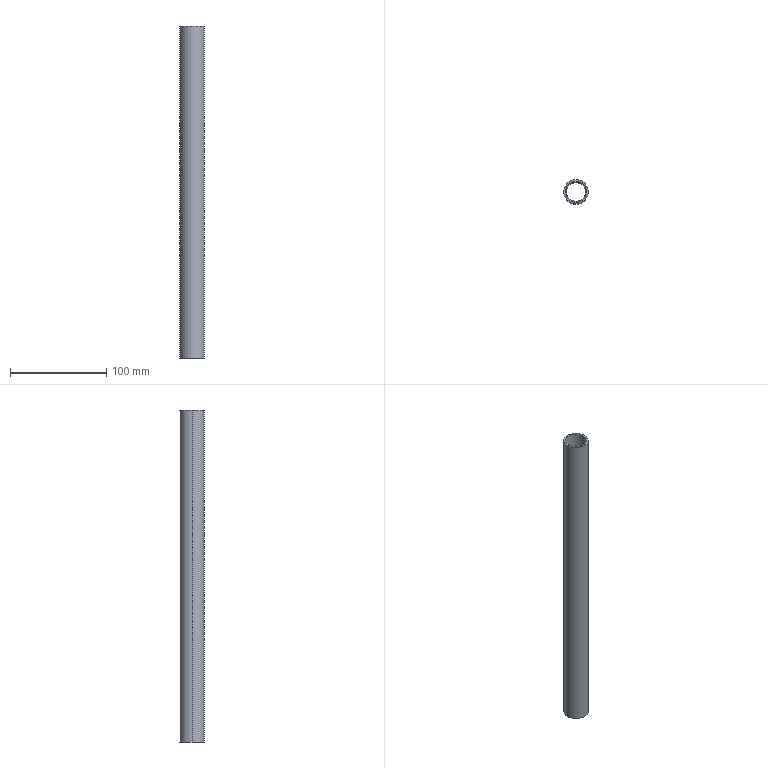Part | STEP file | 31E-01006QY25 | 1 solid | 12 faces | box 25.4 x 25.4 x 345 mm | volume 60669 mm3 | cylinder 8 | plane 4 | commonest cylinder face diameters 22.2 x4 19.8 x2 25.4 x2
STEP:
#1=CARTESIAN_POINT('',(12.7,0.,0.));
#2=VERTEX_POINT('',#1);
#3=CARTESIAN_POINT('',(12.7,0.,345.));
#4=VERTEX_POINT('',#3);
#5=CARTESIAN_POINT('',(12.7,0.,172.5));
#6=DIRECTION('',(0.,0.,1.));
#7=VECTOR('',#6,1.);
#8=LINE('',#5,#7);
#9=EDGE_CURVE('',#2,#4,#8,.T.);
#10=ORIENTED_EDGE('',*,*,#9,.F.);
#11=CARTESIAN_POINT('',(-12.7,0.,0.));
#12=VERTEX_POINT('',#11);
#13=CARTESIAN_POINT('',(0.,0.,0.));
#14=DIRECTION('',(0.,0.,1.));
#15=AXIS2_PLACEMENT_3D('',#13,#14,$);
#16=CIRCLE('',#15,12.7);
#17=EDGE_CURVE('',#2,#12,#16,.T.);
#18=ORIENTED_EDGE('',*,*,#17,.T.);
#19=CARTESIAN_POINT('',(-12.7,0.,345.));
#20=VERTEX_POINT('',#19);
#21=CARTESIAN_POINT('',(-12.7,0.,172.5));
#22=DIRECTION('',(0.,0.,1.));
#23=VECTOR('',#22,1.);
#24=LINE('',#21,#23);
#25=EDGE_CURVE('',#12,#20,#24,.T.);
#26=ORIENTED_EDGE('',*,*,#25,.T.);
#27=CARTESIAN_POINT('',(0.,0.,345.));
#28=DIRECTION('',(0.,0.,1.));
#29=AXIS2_PLACEMENT_3D('',#27,#28,$);
#30=CIRCLE('',#29,12.7);
#31=EDGE_CURVE('',#4,#20,#30,.T.);
#32=ORIENTED_EDGE('',*,*,#31,.F.);
#33=EDGE_LOOP('',(#10,#18,#26,#32));
#34=FACE_OUTER_BOUND('',#33,.T.);
#35=CARTESIAN_POINT('',(0.,0.,172.5));
#36=DIRECTION('',(0.,0.,1.));
#37=DIRECTION('',(1.,0.,0.));
#38=AXIS2_PLACEMENT_3D('',#35,#36,#37);
#39=CYLINDRICAL_SURFACE('',#38,12.7);
#40=ADVANCED_FACE('',(#34),#39,.T.);
#41=ORIENTED_EDGE('',*,*,#25,.F.);
#42=CARTESIAN_POINT('',(0.,0.,0.));
#43=DIRECTION('',(0.,0.,1.));
#44=AXIS2_PLACEMENT_3D('',#42,#43,$);
#45=CIRCLE('',#44,12.7);
#46=EDGE_CURVE('',#12,#2,#45,.T.);
#47=ORIENTED_EDGE('',*,*,#46,.T.);
#48=ORIENTED_EDGE('',*,*,#9,.T.);
#49=CARTESIAN_POINT('',(0.,0.,345.));
#50=DIRECTION('',(0.,0.,1.));
#51=AXIS2_PLACEMENT_3D('',#49,#50,$);
#52=CIRCLE('',#51,12.7);
#53=EDGE_CURVE('',#20,#4,#52,.T.);
#54=ORIENTED_EDGE('',*,*,#53,.F.);
#55=EDGE_LOOP('',(#41,#47,#48,#54));
#56=FACE_OUTER_BOUND('',#55,.T.);
#57=ADVANCED_FACE('',(#56),#39,.T.);
#58=ORIENTED_EDGE('',*,*,#31,.T.);
#59=ORIENTED_EDGE('',*,*,#53,.T.);
#60=EDGE_LOOP('',(#58,#59));
#61=FACE_OUTER_BOUND('',#60,.T.);
#62=CARTESIAN_POINT('',(11.1,0.,345.));
#63=VERTEX_POINT('',#62);
#64=CARTESIAN_POINT('',(-11.1,0.,345.));
#65=VERTEX_POINT('',#64);
#66=CARTESIAN_POINT('',(0.,0.,345.));
#67=DIRECTION('',(0.,0.,1.));
#68=AXIS2_PLACEMENT_3D('',#66,#67,$);
#69=CIRCLE('',#68,11.1);
#70=EDGE_CURVE('',#63,#65,#69,.T.);
#71=ORIENTED_EDGE('',*,*,#70,.F.);
#72=CARTESIAN_POINT('',(0.,0.,345.));
#73=DIRECTION('',(0.,0.,1.));
#74=AXIS2_PLACEMENT_3D('',#72,#73,$);
#75=CIRCLE('',#74,11.1);
#76=EDGE_CURVE('',#65,#63,#75,.T.);
#77=ORIENTED_EDGE('',*,*,#76,.F.);
#78=EDGE_LOOP('',(#71,#77));
#79=FACE_BOUND('',#78,.T.);
#80=CARTESIAN_POINT('',(0.,0.,345.));
#81=DIRECTION('',(0.,0.,1.));
#82=DIRECTION('',(1.,0.,0.));
#83=AXIS2_PLACEMENT_3D('',#80,#81,#82);
#84=PLANE('',#83);
#85=ADVANCED_FACE('',(#61,#79),#84,.T.);
#86=CARTESIAN_POINT('',(11.1,0.,295.));
#87=VERTEX_POINT('',#86);
#88=CARTESIAN_POINT('',(11.1,0.,172.5));
#89=DIRECTION('',(0.,0.,1.));
#90=VECTOR('',#89,1.);
#91=LINE('',#88,#90);
#92=EDGE_CURVE('',#63,#87,#91,.F.);
#93=ORIENTED_EDGE('',*,*,#92,.F.);
#94=ORIENTED_EDGE('',*,*,#70,.T.);
#95=CARTESIAN_POINT('',(-11.1,0.,295.));
#96=VERTEX_POINT('',#95);
#97=CARTESIAN_POINT('',(-11.1,0.,172.5));
#98=DIRECTION('',(0.,0.,1.));
#99=VECTOR('',#98,1.);
#100=LINE('',#97,#99);
#101=EDGE_CURVE('',#65,#96,#100,.F.);
#102=ORIENTED_EDGE('',*,*,#101,.T.);
#103=CARTESIAN_POINT('',(0.,0.,295.));
#104=DIRECTION('',(0.,0.,1.));
#105=AXIS2_PLACEMENT_3D('',#103,#104,$);
#106=CIRCLE('',#105,11.1);
#107=EDGE_CURVE('',#87,#96,#106,.T.);
#108=ORIENTED_EDGE('',*,*,#107,.F.);
#109=EDGE_LOOP('',(#93,#94,#102,#108));
#110=FACE_OUTER_BOUND('',#109,.T.);
#111=CARTESIAN_POINT('',(0.,0.,320.));
#112=DIRECTION('',(0.,0.,1.));
#113=DIRECTION('',(1.,0.,0.));
#114=AXIS2_PLACEMENT_3D('',#111,#112,#113);
#115=CYLINDRICAL_SURFACE('',#114,11.1);
#116=ADVANCED_FACE('',(#110),#115,.F.);
#117=ORIENTED_EDGE('',*,*,#101,.F.);
#118=ORIENTED_EDGE('',*,*,#76,.T.);
#119=ORIENTED_EDGE('',*,*,#92,.T.);
#120=CARTESIAN_POINT('',(0.,0.,295.));
#121=DIRECTION('',(0.,0.,1.));
#122=AXIS2_PLACEMENT_3D('',#120,#121,$);
#123=CIRCLE('',#122,11.1);
#124=EDGE_CURVE('',#96,#87,#123,.T.);
#125=ORIENTED_EDGE('',*,*,#124,.F.);
#126=EDGE_LOOP('',(#117,#118,#119,#125));
#127=FACE_OUTER_BOUND('',#126,.T.);
#128=ADVANCED_FACE('',(#127),#115,.F.);
#129=ORIENTED_EDGE('',*,*,#107,.T.);
#130=ORIENTED_EDGE('',*,*,#124,.T.);
#131=EDGE_LOOP('',(#129,#130));
#132=FACE_OUTER_BOUND('',#131,.T.);
#133=CARTESIAN_POINT('',(-9.9,0.,295.));
#134=VERTEX_POINT('',#133);
#135=CARTESIAN_POINT('',(9.9,0.,295.));
#136=VERTEX_POINT('',#135);
#137=CARTESIAN_POINT('',(0.,0.,295.));
#138=DIRECTION('',(0.,0.,1.));
#139=AXIS2_PLACEMENT_3D('',#137,#138,$);
#140=CIRCLE('',#139,9.9);
#141=EDGE_CURVE('',#134,#136,#140,.T.);
#142=ORIENTED_EDGE('',*,*,#141,.F.);
#143=CARTESIAN_POINT('',(0.,0.,295.));
#144=DIRECTION('',(0.,0.,1.));
#145=AXIS2_PLACEMENT_3D('',#143,#144,$);
#146=CIRCLE('',#145,9.9);
#147=EDGE_CURVE('',#136,#134,#146,.T.);
#148=ORIENTED_EDGE('',*,*,#147,.F.);
#149=EDGE_LOOP('',(#142,#148));
#150=FACE_BOUND('',#149,.T.);
#151=CARTESIAN_POINT('',(0.,0.,295.));
#152=DIRECTION('',(0.,0.,1.));
#153=DIRECTION('',(1.,0.,0.));
#154=AXIS2_PLACEMENT_3D('',#151,#152,#153);
#155=PLANE('',#154);
#156=ADVANCED_FACE('',(#132,#150),#155,.T.);
#157=CARTESIAN_POINT('',(-9.9,0.,50.));
#158=VERTEX_POINT('',#157);
#159=CARTESIAN_POINT('',(9.9,0.,50.));
#160=VERTEX_POINT('',#159);
#161=CARTESIAN_POINT('',(0.,0.,50.));
#162=DIRECTION('',(0.,0.,1.));
#163=AXIS2_PLACEMENT_3D('',#161,#162,$);
#164=CIRCLE('',#163,9.9);
#165=EDGE_CURVE('',#158,#160,#164,.T.);
#166=ORIENTED_EDGE('',*,*,#165,.F.);
#167=CARTESIAN_POINT('',(-9.9,0.,172.5));
#168=DIRECTION('',(0.,0.,1.));
#169=VECTOR('',#168,1.);
#170=LINE('',#167,#169);
#171=EDGE_CURVE('',#158,#134,#170,.T.);
#172=ORIENTED_EDGE('',*,*,#171,.T.);
#173=ORIENTED_EDGE('',*,*,#141,.T.);
#174=CARTESIAN_POINT('',(9.9,0.,172.5));
#175=DIRECTION('',(0.,0.,1.));
#176=VECTOR('',#175,1.);
#177=LINE('',#174,#176);
#178=EDGE_CURVE('',#160,#136,#177,.T.);
#179=ORIENTED_EDGE('',*,*,#178,.F.);
#180=EDGE_LOOP('',(#166,#172,#173,#179));
#181=FACE_OUTER_BOUND('',#180,.T.);
#182=CARTESIAN_POINT('',(0.,0.,172.5));
#183=DIRECTION('',(0.,0.,1.));
#184=DIRECTION('',(1.,0.,0.));
#185=AXIS2_PLACEMENT_3D('',#182,#183,#184);
#186=CYLINDRICAL_SURFACE('',#185,9.9);
#187=ADVANCED_FACE('',(#181),#186,.F.);
#188=CARTESIAN_POINT('',(0.,0.,50.));
#189=DIRECTION('',(0.,0.,1.));
#190=AXIS2_PLACEMENT_3D('',#188,#189,$);
#191=CIRCLE('',#190,9.9);
#192=EDGE_CURVE('',#160,#158,#191,.T.);
#193=ORIENTED_EDGE('',*,*,#192,.F.);
#194=ORIENTED_EDGE('',*,*,#178,.T.);
#195=ORIENTED_EDGE('',*,*,#147,.T.);
#196=ORIENTED_EDGE('',*,*,#171,.F.);
#197=EDGE_LOOP('',(#193,#194,#195,#196));
#198=FACE_OUTER_BOUND('',#197,.T.);
#199=ADVANCED_FACE('',(#198),#186,.F.);
#200=ORIENTED_EDGE('',*,*,#46,.F.);
#201=ORIENTED_EDGE('',*,*,#17,.F.);
#202=EDGE_LOOP('',(#200,#201));
#203=FACE_OUTER_BOUND('',#202,.T.);
#204=CARTESIAN_POINT('',(-11.1,0.,0.));
#205=VERTEX_POINT('',#204);
#206=CARTESIAN_POINT('',(11.1,0.,0.));
#207=VERTEX_POINT('',#206);
#208=CARTESIAN_POINT('',(0.,0.,0.));
#209=DIRECTION('',(0.,0.,1.));
#210=AXIS2_PLACEMENT_3D('',#208,#209,$);
#211=CIRCLE('',#210,11.1);
#212=EDGE_CURVE('',#205,#207,#211,.T.);
#213=ORIENTED_EDGE('',*,*,#212,.T.);
#214=CARTESIAN_POINT('',(0.,0.,0.));
#215=DIRECTION('',(0.,0.,1.));
#216=AXIS2_PLACEMENT_3D('',#214,#215,$);
#217=CIRCLE('',#216,11.1);
#218=EDGE_CURVE('',#207,#205,#217,.T.);
#219=ORIENTED_EDGE('',*,*,#218,.T.);
#220=EDGE_LOOP('',(#213,#219));
#221=FACE_BOUND('',#220,.T.);
#222=CARTESIAN_POINT('',(0.,0.,0.));
#223=DIRECTION('',(0.,0.,1.));
#224=DIRECTION('',(1.,0.,0.));
#225=AXIS2_PLACEMENT_3D('',#222,#223,#224);
#226=PLANE('',#225);
#227=ADVANCED_FACE('',(#203,#221),#226,.F.);
#228=CARTESIAN_POINT('',(11.1,0.,50.));
#229=VERTEX_POINT('',#228);
#230=CARTESIAN_POINT('',(-11.1,0.,50.));
#231=VERTEX_POINT('',#230);
#232=CARTESIAN_POINT('',(0.,0.,50.));
#233=DIRECTION('',(0.,0.,1.));
#234=AXIS2_PLACEMENT_3D('',#232,#233,$);
#235=CIRCLE('',#234,11.1);
#236=EDGE_CURVE('',#229,#231,#235,.T.);
#237=ORIENTED_EDGE('',*,*,#236,.T.);
#238=CARTESIAN_POINT('',(-11.1,0.,172.5));
#239=DIRECTION('',(0.,0.,1.));
#240=VECTOR('',#239,1.);
#241=LINE('',#238,#240);
#242=EDGE_CURVE('',#205,#231,#241,.T.);
#243=ORIENTED_EDGE('',*,*,#242,.F.);
#244=ORIENTED_EDGE('',*,*,#218,.F.);
#245=CARTESIAN_POINT('',(11.1,0.,172.5));
#246=DIRECTION('',(0.,0.,1.));
#247=VECTOR('',#246,1.);
#248=LINE('',#245,#247);
#249=EDGE_CURVE('',#207,#229,#248,.T.);
#250=ORIENTED_EDGE('',*,*,#249,.T.);
#251=EDGE_LOOP('',(#237,#243,#244,#250));
#252=FACE_OUTER_BOUND('',#251,.T.);
#253=ADVANCED_FACE('',(#252),#115,.F.);
#254=CARTESIAN_POINT('',(0.,0.,50.));
#255=DIRECTION('',(0.,0.,1.));
#256=AXIS2_PLACEMENT_3D('',#254,#255,$);
#257=CIRCLE('',#256,11.1);
#258=EDGE_CURVE('',#231,#229,#257,.T.);
#259=ORIENTED_EDGE('',*,*,#258,.T.);
#260=ORIENTED_EDGE('',*,*,#249,.F.);
#261=ORIENTED_EDGE('',*,*,#212,.F.);
#262=ORIENTED_EDGE('',*,*,#242,.T.);
#263=EDGE_LOOP('',(#259,#260,#261,#262));
#264=FACE_OUTER_BOUND('',#263,.T.);
#265=ADVANCED_FACE('',(#264),#115,.F.);
#266=ORIENTED_EDGE('',*,*,#258,.F.);
#267=ORIENTED_EDGE('',*,*,#236,.F.);
#268=EDGE_LOOP('',(#266,#267));
#269=FACE_OUTER_BOUND('',#268,.T.);
#270=ORIENTED_EDGE('',*,*,#165,.T.);
#271=ORIENTED_EDGE('',*,*,#192,.T.);
#272=EDGE_LOOP('',(#270,#271));
#273=FACE_BOUND('',#272,.T.);
#274=CARTESIAN_POINT('',(0.,0.,50.));
#275=DIRECTION('',(0.,0.,1.));
#276=DIRECTION('',(1.,0.,0.));
#277=AXIS2_PLACEMENT_3D('',#274,#275,#276);
#278=PLANE('',#277);
#279=ADVANCED_FACE('',(#269,#273),#278,.F.);
#280=CLOSED_SHELL('',(#40,#57,#85,#116,#128,#156,#187,#199,#227,#253,#265,#279));
#281=MANIFOLD_SOLID_BREP('',#280);
#282=(LENGTH_UNIT()NAMED_UNIT(*)SI_UNIT(.MILLI.,.METRE.));
#283=UNCERTAINTY_MEASURE_WITH_UNIT(LENGTH_MEASURE(0.005),#282,'','');
#284=(NAMED_UNIT(*)PLANE_ANGLE_UNIT()SI_UNIT($,.RADIAN.));
#285=(NAMED_UNIT(*)SI_UNIT($,.STERADIAN.)SOLID_ANGLE_UNIT());
#286=(GEOMETRIC_REPRESENTATION_CONTEXT(3)GLOBAL_UNCERTAINTY_ASSIGNED_CONTEXT((#283))GLOBAL_UNIT_ASSIGNED_CONTEXT((#282,#284,#285))REPRESENTATION_CONTEXT('',''));
#287=ADVANCED_BREP_SHAPE_REPRESENTATION('',(#281),#286);